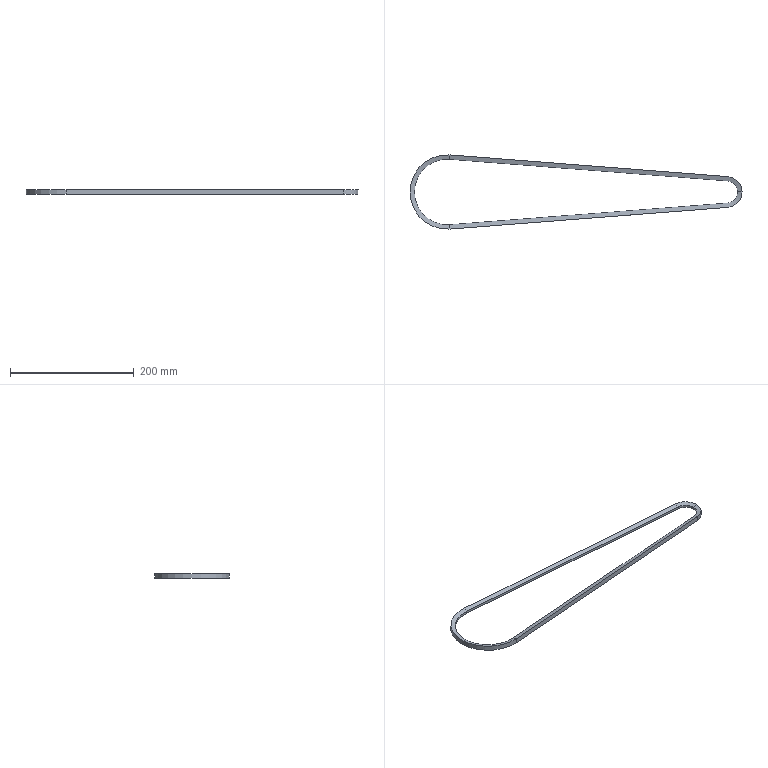Part | NX | features BREP 1 | 1 solid | 18 faces | box 535.87 x 119.96 x 8 mm | volume 48380 mm3 | plane 8 | cone 6 | cylinder 4 | commonest cylinder face diameters 35.96 x1 49.96 x1 105.96 x1 119.96 x1
STEP:
#1=CARTESIAN_POINT('',(4.112,52.82,-2.));
#2=VERTEX_POINT('',#1);
#3=CARTESIAN_POINT('',(-52.98,0.,-2.));
#4=VERTEX_POINT('',#3);
#5=CARTESIAN_POINT('',(0.,0.,-2.));
#6=DIRECTION('',(0.,0.,1.));
#7=DIRECTION('',(1.,0.,0.));
#8=AXIS2_PLACEMENT_3D('',#5,#6,#7);
#9=CIRCLE('',#8,52.98);
#10=EDGE_CURVE('',#2,#4,#9,.T.);
#11=ORIENTED_EDGE('',*,*,#10,.T.);
#12=CARTESIAN_POINT('',(-59.98,0.,-4.));
#13=VERTEX_POINT('',#12);
#14=CARTESIAN_POINT('',(-52.98,0.,-2.));
#15=DIRECTION('',(-0.9615,0.,-0.2747));
#16=VECTOR('',#15,1000.);
#17=LINE('',#14,#16);
#18=EDGE_CURVE('',#4,#13,#17,.T.);
#19=ORIENTED_EDGE('',*,*,#18,.T.);
#20=CARTESIAN_POINT('',(4.656,59.799,-4.));
#21=VERTEX_POINT('',#20);
#22=CARTESIAN_POINT('',(0.,0.,-4.));
#23=DIRECTION('',(0.,0.,1.));
#24=DIRECTION('',(1.,0.,0.));
#25=AXIS2_PLACEMENT_3D('',#22,#23,#24);
#26=CIRCLE('',#25,59.98);
#27=EDGE_CURVE('',#21,#13,#26,.T.);
#28=ORIENTED_EDGE('',*,*,#27,.F.);
#29=CARTESIAN_POINT('',(4.112,52.82,-2.));
#30=DIRECTION('',(0.07463,0.9586,-0.2747));
#31=VECTOR('',#30,1000.);
#32=LINE('',#29,#31);
#33=EDGE_CURVE('',#2,#21,#32,.T.);
#34=ORIENTED_EDGE('',*,*,#33,.F.);
#35=EDGE_LOOP('',(#11,#19,#28,#34));
#36=FACE_BOUND('',#35,.T.);
#37=CARTESIAN_POINT('',(0.,0.,-2.));
#38=DIRECTION('',(0.,0.,-1.));
#39=DIRECTION('',(1.,0.,0.));
#40=AXIS2_PLACEMENT_3D('',#37,#38,#39);
#41=CONICAL_SURFACE('',#40,52.98,1.292);
#42=ADVANCED_FACE('',(#36),#41,.F.);
#43=CARTESIAN_POINT('',(452.306,17.926,2.));
#44=VERTEX_POINT('',#43);
#45=CARTESIAN_POINT('',(468.89,0.,2.));
#46=VERTEX_POINT('',#45);
#47=CARTESIAN_POINT('',(450.91,0.,2.));
#48=DIRECTION('',(0.,0.,-1.));
#49=DIRECTION('',(-1.,0.,0.));
#50=AXIS2_PLACEMENT_3D('',#47,#48,#49);
#51=CIRCLE('',#50,17.98);
#52=EDGE_CURVE('',#44,#46,#51,.T.);
#53=ORIENTED_EDGE('',*,*,#52,.T.);
#54=CARTESIAN_POINT('',(475.89,0.,4.));
#55=VERTEX_POINT('',#54);
#56=CARTESIAN_POINT('',(475.89,0.,4.));
#57=DIRECTION('',(0.9615,0.,0.2747));
#58=VECTOR('',#57,1000.);
#59=LINE('',#56,#58);
#60=EDGE_CURVE('',#46,#55,#59,.T.);
#61=ORIENTED_EDGE('',*,*,#60,.T.);
#62=CARTESIAN_POINT('',(452.849,24.905,4.));
#63=VERTEX_POINT('',#62);
#64=CARTESIAN_POINT('',(450.91,0.,4.));
#65=DIRECTION('',(0.,0.,-1.));
#66=DIRECTION('',(-1.,0.,0.));
#67=AXIS2_PLACEMENT_3D('',#64,#65,#66);
#68=CIRCLE('',#67,24.98);
#69=EDGE_CURVE('',#63,#55,#68,.T.);
#70=ORIENTED_EDGE('',*,*,#69,.F.);
#71=CARTESIAN_POINT('',(452.306,17.926,2.));
#72=DIRECTION('',(-0.07463,-0.9586,-0.2747));
#73=VECTOR('',#72,1000.);
#74=LINE('',#71,#73);
#75=EDGE_CURVE('',#63,#44,#74,.T.);
#76=ORIENTED_EDGE('',*,*,#75,.T.);
#77=EDGE_LOOP('',(#53,#61,#70,#76));
#78=FACE_BOUND('',#77,.T.);
#79=CARTESIAN_POINT('',(450.91,0.,4.));
#80=DIRECTION('',(0.,0.,1.));
#81=DIRECTION('',(-1.,0.,0.));
#82=AXIS2_PLACEMENT_3D('',#79,#80,#81);
#83=CONICAL_SURFACE('',#82,24.98,1.292);
#84=ADVANCED_FACE('',(#78),#83,.F.);
#85=CARTESIAN_POINT('',(452.306,-17.926,2.));
#86=VERTEX_POINT('',#85);
#87=CARTESIAN_POINT('',(452.306,-17.926,-2.));
#88=VERTEX_POINT('',#87);
#89=CARTESIAN_POINT('',(452.306,-17.926,2.));
#90=DIRECTION('',(0.,0.,-1.));
#91=VECTOR('',#90,1000.);
#92=LINE('',#89,#91);
#93=EDGE_CURVE('',#86,#88,#92,.T.);
#94=ORIENTED_EDGE('',*,*,#93,.T.);
#95=CARTESIAN_POINT('',(4.112,-52.82,-2.));
#96=VERTEX_POINT('',#95);
#97=CARTESIAN_POINT('',(452.306,-17.926,-2.));
#98=DIRECTION('',(-0.997,-0.07762,0.));
#99=VECTOR('',#98,1000.);
#100=LINE('',#97,#99);
#101=EDGE_CURVE('',#88,#96,#100,.T.);
#102=ORIENTED_EDGE('',*,*,#101,.T.);
#103=CARTESIAN_POINT('',(4.112,-52.82,2.));
#104=VERTEX_POINT('',#103);
#105=CARTESIAN_POINT('',(4.112,-52.82,2.));
#106=DIRECTION('',(0.,0.,-1.));
#107=VECTOR('',#106,1000.);
#108=LINE('',#105,#107);
#109=EDGE_CURVE('',#104,#96,#108,.T.);
#110=ORIENTED_EDGE('',*,*,#109,.F.);
#111=CARTESIAN_POINT('',(452.306,-17.926,2.));
#112=DIRECTION('',(-0.997,-0.07762,0.));
#113=VECTOR('',#112,1000.);
#114=LINE('',#111,#113);
#115=EDGE_CURVE('',#86,#104,#114,.T.);
#116=ORIENTED_EDGE('',*,*,#115,.F.);
#117=EDGE_LOOP('',(#94,#102,#110,#116));
#118=FACE_BOUND('',#117,.T.);
#119=CARTESIAN_POINT('',(452.306,-17.926,2.));
#120=DIRECTION('',(-0.07762,0.997,0.));
#121=DIRECTION('',(0.,0.,-1.));
#122=AXIS2_PLACEMENT_3D('',#119,#120,#121);
#123=PLANE('',#122);
#124=ADVANCED_FACE('',(#118),#123,.T.);
#125=CARTESIAN_POINT('',(452.849,-24.905,-4.));
#126=VERTEX_POINT('',#125);
#127=CARTESIAN_POINT('',(452.306,-17.926,-2.));
#128=DIRECTION('',(0.07463,-0.9586,-0.2747));
#129=VECTOR('',#128,1000.);
#130=LINE('',#127,#129);
#131=EDGE_CURVE('',#88,#126,#130,.T.);
#132=ORIENTED_EDGE('',*,*,#131,.T.);
#133=CARTESIAN_POINT('',(4.656,-59.799,-4.));
#134=VERTEX_POINT('',#133);
#135=CARTESIAN_POINT('',(452.849,-24.905,-4.));
#136=DIRECTION('',(-0.997,-0.07762,0.));
#137=VECTOR('',#136,1000.);
#138=LINE('',#135,#137);
#139=EDGE_CURVE('',#126,#134,#138,.T.);
#140=ORIENTED_EDGE('',*,*,#139,.T.);
#141=CARTESIAN_POINT('',(4.112,-52.82,-2.));
#142=DIRECTION('',(0.07463,-0.9586,-0.2747));
#143=VECTOR('',#142,1000.);
#144=LINE('',#141,#143);
#145=EDGE_CURVE('',#96,#134,#144,.T.);
#146=ORIENTED_EDGE('',*,*,#145,.F.);
#147=ORIENTED_EDGE('',*,*,#101,.F.);
#148=EDGE_LOOP('',(#132,#140,#146,#147));
#149=FACE_BOUND('',#148,.T.);
#150=CARTESIAN_POINT('',(452.306,-17.926,-2.));
#151=DIRECTION('',(-0.02132,0.2739,-0.9615));
#152=DIRECTION('',(0.9998,0.,-0.02217));
#153=AXIS2_PLACEMENT_3D('',#150,#151,#152);
#154=PLANE('',#153);
#155=ADVANCED_FACE('',(#149),#154,.T.);
#156=CARTESIAN_POINT('',(452.849,-24.905,4.));
#157=VERTEX_POINT('',#156);
#158=CARTESIAN_POINT('',(452.849,-24.905,-4.));
#159=DIRECTION('',(0.,0.,1.));
#160=VECTOR('',#159,1000.);
#161=LINE('',#158,#160);
#162=EDGE_CURVE('',#126,#157,#161,.T.);
#163=ORIENTED_EDGE('',*,*,#162,.T.);
#164=CARTESIAN_POINT('',(4.656,-59.799,4.));
#165=VERTEX_POINT('',#164);
#166=CARTESIAN_POINT('',(452.849,-24.905,4.));
#167=DIRECTION('',(-0.997,-0.07762,0.));
#168=VECTOR('',#167,1000.);
#169=LINE('',#166,#168);
#170=EDGE_CURVE('',#157,#165,#169,.T.);
#171=ORIENTED_EDGE('',*,*,#170,.T.);
#172=CARTESIAN_POINT('',(4.656,-59.799,-4.));
#173=DIRECTION('',(0.,0.,1.));
#174=VECTOR('',#173,1000.);
#175=LINE('',#172,#174);
#176=EDGE_CURVE('',#134,#165,#175,.T.);
#177=ORIENTED_EDGE('',*,*,#176,.F.);
#178=ORIENTED_EDGE('',*,*,#139,.F.);
#179=EDGE_LOOP('',(#163,#171,#177,#178));
#180=FACE_BOUND('',#179,.T.);
#181=CARTESIAN_POINT('',(452.849,-24.905,-4.));
#182=DIRECTION('',(0.07762,-0.997,0.));
#183=DIRECTION('',(0.,0.,1.));
#184=AXIS2_PLACEMENT_3D('',#181,#182,#183);
#185=PLANE('',#184);
#186=ADVANCED_FACE('',(#180),#185,.T.);
#187=CARTESIAN_POINT('',(452.306,-17.926,2.));
#188=DIRECTION('',(-0.07463,0.9586,-0.2747));
#189=VECTOR('',#188,1000.);
#190=LINE('',#187,#189);
#191=EDGE_CURVE('',#157,#86,#190,.T.);
#192=ORIENTED_EDGE('',*,*,#191,.T.);
#193=ORIENTED_EDGE('',*,*,#115,.T.);
#194=CARTESIAN_POINT('',(4.112,-52.82,2.));
#195=DIRECTION('',(-0.07463,0.9586,-0.2747));
#196=VECTOR('',#195,1000.);
#197=LINE('',#194,#196);
#198=EDGE_CURVE('',#165,#104,#197,.T.);
#199=ORIENTED_EDGE('',*,*,#198,.F.);
#200=ORIENTED_EDGE('',*,*,#170,.F.);
#201=EDGE_LOOP('',(#192,#193,#199,#200));
#202=FACE_BOUND('',#201,.T.);
#203=CARTESIAN_POINT('',(452.306,-17.926,2.));
#204=DIRECTION('',(-0.02132,0.2739,0.9615));
#205=DIRECTION('',(-0.997,-0.07762,0.));
#206=AXIS2_PLACEMENT_3D('',#203,#204,#205);
#207=PLANE('',#206);
#208=ADVANCED_FACE('',(#202),#207,.T.);
#209=CARTESIAN_POINT('',(452.306,17.926,-2.));
#210=VERTEX_POINT('',#209);
#211=CARTESIAN_POINT('',(452.306,17.926,2.));
#212=DIRECTION('',(0.,0.,-1.));
#213=VECTOR('',#212,1000.);
#214=LINE('',#211,#213);
#215=EDGE_CURVE('',#44,#210,#214,.T.);
#216=ORIENTED_EDGE('',*,*,#215,.T.);
#217=CARTESIAN_POINT('',(450.91,0.,-2.));
#218=DIRECTION('',(0.,0.,-1.));
#219=DIRECTION('',(-1.,0.,0.));
#220=AXIS2_PLACEMENT_3D('',#217,#218,#219);
#221=CIRCLE('',#220,17.98);
#222=EDGE_CURVE('',#210,#88,#221,.T.);
#223=ORIENTED_EDGE('',*,*,#222,.T.);
#224=ORIENTED_EDGE('',*,*,#93,.F.);
#225=CARTESIAN_POINT('',(450.91,0.,2.));
#226=DIRECTION('',(0.,0.,-1.));
#227=DIRECTION('',(-1.,0.,0.));
#228=AXIS2_PLACEMENT_3D('',#225,#226,#227);
#229=CIRCLE('',#228,17.98);
#230=EDGE_CURVE('',#46,#86,#229,.T.);
#231=ORIENTED_EDGE('',*,*,#230,.F.);
#232=ORIENTED_EDGE('',*,*,#52,.F.);
#233=EDGE_LOOP('',(#216,#223,#224,#231,#232));
#234=FACE_BOUND('',#233,.T.);
#235=CARTESIAN_POINT('',(450.91,0.,0.));
#236=DIRECTION('',(0.,0.,-1.));
#237=DIRECTION('',(1.,0.,0.));
#238=AXIS2_PLACEMENT_3D('',#235,#236,#237);
#239=CYLINDRICAL_SURFACE('',#238,17.98);
#240=ADVANCED_FACE('',(#234),#239,.F.);
#241=CARTESIAN_POINT('',(452.849,24.905,-4.));
#242=VERTEX_POINT('',#241);
#243=CARTESIAN_POINT('',(452.306,17.926,-2.));
#244=DIRECTION('',(0.07463,0.9586,-0.2747));
#245=VECTOR('',#244,1000.);
#246=LINE('',#243,#245);
#247=EDGE_CURVE('',#210,#242,#246,.T.);
#248=ORIENTED_EDGE('',*,*,#247,.T.);
#249=CARTESIAN_POINT('',(450.91,0.,-4.));
#250=DIRECTION('',(0.,0.,-1.));
#251=DIRECTION('',(-1.,0.,0.));
#252=AXIS2_PLACEMENT_3D('',#249,#250,#251);
#253=CIRCLE('',#252,24.98);
#254=EDGE_CURVE('',#242,#126,#253,.T.);
#255=ORIENTED_EDGE('',*,*,#254,.T.);
#256=ORIENTED_EDGE('',*,*,#131,.F.);
#257=ORIENTED_EDGE('',*,*,#222,.F.);
#258=EDGE_LOOP('',(#248,#255,#256,#257));
#259=FACE_BOUND('',#258,.T.);
#260=CARTESIAN_POINT('',(450.91,0.,-2.));
#261=DIRECTION('',(0.,0.,-1.));
#262=DIRECTION('',(1.,0.,0.));
#263=AXIS2_PLACEMENT_3D('',#260,#261,#262);
#264=CONICAL_SURFACE('',#263,17.98,1.292);
#265=ADVANCED_FACE('',(#259),#264,.F.);
#266=CARTESIAN_POINT('',(452.849,24.905,-4.));
#267=DIRECTION('',(0.,0.,1.));
#268=VECTOR('',#267,1000.);
#269=LINE('',#266,#268);
#270=EDGE_CURVE('',#242,#63,#269,.T.);
#271=ORIENTED_EDGE('',*,*,#270,.T.);
#272=ORIENTED_EDGE('',*,*,#69,.T.);
#273=CARTESIAN_POINT('',(450.91,0.,4.));
#274=DIRECTION('',(0.,0.,-1.));
#275=DIRECTION('',(-1.,0.,0.));
#276=AXIS2_PLACEMENT_3D('',#273,#274,#275);
#277=CIRCLE('',#276,24.98);
#278=EDGE_CURVE('',#55,#157,#277,.T.);
#279=ORIENTED_EDGE('',*,*,#278,.T.);
#280=ORIENTED_EDGE('',*,*,#162,.F.);
#281=ORIENTED_EDGE('',*,*,#254,.F.);
#282=EDGE_LOOP('',(#271,#272,#279,#280,#281));
#283=FACE_BOUND('',#282,.T.);
#284=CARTESIAN_POINT('',(450.91,0.,0.));
#285=DIRECTION('',(0.,0.,-1.));
#286=DIRECTION('',(1.,0.,0.));
#287=AXIS2_PLACEMENT_3D('',#284,#285,#286);
#288=CYLINDRICAL_SURFACE('',#287,24.98);
#289=ADVANCED_FACE('',(#283),#288,.T.);
#290=ORIENTED_EDGE('',*,*,#60,.F.);
#291=ORIENTED_EDGE('',*,*,#230,.T.);
#292=ORIENTED_EDGE('',*,*,#191,.F.);
#293=ORIENTED_EDGE('',*,*,#278,.F.);
#294=EDGE_LOOP('',(#290,#291,#292,#293));
#295=FACE_BOUND('',#294,.T.);
#296=CARTESIAN_POINT('',(450.91,0.,4.));
#297=DIRECTION('',(0.,0.,1.));
#298=DIRECTION('',(-1.,0.,0.));
#299=AXIS2_PLACEMENT_3D('',#296,#297,#298);
#300=CONICAL_SURFACE('',#299,24.98,1.292);
#301=ADVANCED_FACE('',(#295),#300,.F.);
#302=CARTESIAN_POINT('',(4.112,52.82,2.));
#303=VERTEX_POINT('',#302);
#304=CARTESIAN_POINT('',(4.112,52.82,2.));
#305=DIRECTION('',(0.,0.,-1.));
#306=VECTOR('',#305,1000.);
#307=LINE('',#304,#306);
#308=EDGE_CURVE('',#303,#2,#307,.T.);
#309=ORIENTED_EDGE('',*,*,#308,.T.);
#310=CARTESIAN_POINT('',(4.112,52.82,-2.));
#311=DIRECTION('',(0.997,-0.07762,0.));
#312=VECTOR('',#311,1000.);
#313=LINE('',#310,#312);
#314=EDGE_CURVE('',#2,#210,#313,.T.);
#315=ORIENTED_EDGE('',*,*,#314,.T.);
#316=ORIENTED_EDGE('',*,*,#215,.F.);
#317=CARTESIAN_POINT('',(4.112,52.82,2.));
#318=DIRECTION('',(0.997,-0.07762,0.));
#319=VECTOR('',#318,1000.);
#320=LINE('',#317,#319);
#321=EDGE_CURVE('',#303,#44,#320,.T.);
#322=ORIENTED_EDGE('',*,*,#321,.F.);
#323=EDGE_LOOP('',(#309,#315,#316,#322));
#324=FACE_BOUND('',#323,.T.);
#325=CARTESIAN_POINT('',(4.112,52.82,2.));
#326=DIRECTION('',(-0.07762,-0.997,0.));
#327=DIRECTION('',(0.997,-0.07762,0.));
#328=AXIS2_PLACEMENT_3D('',#325,#326,#327);
#329=PLANE('',#328);
#330=ADVANCED_FACE('',(#324),#329,.T.);
#331=ORIENTED_EDGE('',*,*,#33,.T.);
#332=CARTESIAN_POINT('',(4.656,59.799,-4.));
#333=DIRECTION('',(0.997,-0.07762,0.));
#334=VECTOR('',#333,1000.);
#335=LINE('',#332,#334);
#336=EDGE_CURVE('',#21,#242,#335,.T.);
#337=ORIENTED_EDGE('',*,*,#336,.T.);
#338=ORIENTED_EDGE('',*,*,#247,.F.);
#339=ORIENTED_EDGE('',*,*,#314,.F.);
#340=EDGE_LOOP('',(#331,#337,#338,#339));
#341=FACE_BOUND('',#340,.T.);
#342=CARTESIAN_POINT('',(4.112,52.82,-2.));
#343=DIRECTION('',(-0.02132,-0.2739,-0.9615));
#344=DIRECTION('',(0.,0.9617,-0.274));
#345=AXIS2_PLACEMENT_3D('',#342,#343,#344);
#346=PLANE('',#345);
#347=ADVANCED_FACE('',(#341),#346,.T.);
#348=CARTESIAN_POINT('',(4.656,59.799,4.));
#349=VERTEX_POINT('',#348);
#350=CARTESIAN_POINT('',(4.656,59.799,-4.));
#351=DIRECTION('',(0.,0.,1.));
#352=VECTOR('',#351,1000.);
#353=LINE('',#350,#352);
#354=EDGE_CURVE('',#21,#349,#353,.T.);
#355=ORIENTED_EDGE('',*,*,#354,.T.);
#356=CARTESIAN_POINT('',(4.656,59.799,4.));
#357=DIRECTION('',(0.997,-0.07762,0.));
#358=VECTOR('',#357,1000.);
#359=LINE('',#356,#358);
#360=EDGE_CURVE('',#349,#63,#359,.T.);
#361=ORIENTED_EDGE('',*,*,#360,.T.);
#362=ORIENTED_EDGE('',*,*,#270,.F.);
#363=ORIENTED_EDGE('',*,*,#336,.F.);
#364=EDGE_LOOP('',(#355,#361,#362,#363));
#365=FACE_BOUND('',#364,.T.);
#366=CARTESIAN_POINT('',(4.656,59.799,-4.));
#367=DIRECTION('',(0.07762,0.997,0.));
#368=DIRECTION('',(0.,0.,1.));
#369=AXIS2_PLACEMENT_3D('',#366,#367,#368);
#370=PLANE('',#369);
#371=ADVANCED_FACE('',(#365),#370,.T.);
#372=CARTESIAN_POINT('',(4.112,52.82,2.));
#373=DIRECTION('',(-0.07463,-0.9586,-0.2747));
#374=VECTOR('',#373,1000.);
#375=LINE('',#372,#374);
#376=EDGE_CURVE('',#349,#303,#375,.T.);
#377=ORIENTED_EDGE('',*,*,#376,.T.);
#378=ORIENTED_EDGE('',*,*,#321,.T.);
#379=ORIENTED_EDGE('',*,*,#75,.F.);
#380=ORIENTED_EDGE('',*,*,#360,.F.);
#381=EDGE_LOOP('',(#377,#378,#379,#380));
#382=FACE_BOUND('',#381,.T.);
#383=CARTESIAN_POINT('',(4.112,52.82,2.));
#384=DIRECTION('',(-0.02132,-0.2739,0.9615));
#385=DIRECTION('',(0.997,-0.07762,0.));
#386=AXIS2_PLACEMENT_3D('',#383,#384,#385);
#387=PLANE('',#386);
#388=ADVANCED_FACE('',(#382),#387,.T.);
#389=CARTESIAN_POINT('',(0.,0.,2.));
#390=DIRECTION('',(0.,0.,1.));
#391=DIRECTION('',(1.,0.,0.));
#392=AXIS2_PLACEMENT_3D('',#389,#390,#391);
#393=CIRCLE('',#392,52.98);
#394=EDGE_CURVE('',#303,#104,#393,.T.);
#395=ORIENTED_EDGE('',*,*,#394,.F.);
#396=ORIENTED_EDGE('',*,*,#376,.F.);
#397=CARTESIAN_POINT('',(0.,0.,4.));
#398=DIRECTION('',(0.,0.,1.));
#399=DIRECTION('',(1.,0.,0.));
#400=AXIS2_PLACEMENT_3D('',#397,#398,#399);
#401=CIRCLE('',#400,59.98);
#402=EDGE_CURVE('',#349,#165,#401,.T.);
#403=ORIENTED_EDGE('',*,*,#402,.T.);
#404=ORIENTED_EDGE('',*,*,#198,.T.);
#405=EDGE_LOOP('',(#395,#396,#403,#404));
#406=FACE_BOUND('',#405,.T.);
#407=CARTESIAN_POINT('',(0.,0.,4.));
#408=DIRECTION('',(0.,0.,1.));
#409=DIRECTION('',(-1.,0.,0.));
#410=AXIS2_PLACEMENT_3D('',#407,#408,#409);
#411=CONICAL_SURFACE('',#410,59.98,1.292);
#412=ADVANCED_FACE('',(#406),#411,.F.);
#413=ORIENTED_EDGE('',*,*,#10,.F.);
#414=ORIENTED_EDGE('',*,*,#308,.F.);
#415=ORIENTED_EDGE('',*,*,#394,.T.);
#416=ORIENTED_EDGE('',*,*,#109,.T.);
#417=CARTESIAN_POINT('',(0.,0.,-2.));
#418=DIRECTION('',(0.,0.,1.));
#419=DIRECTION('',(1.,0.,0.));
#420=AXIS2_PLACEMENT_3D('',#417,#418,#419);
#421=CIRCLE('',#420,52.98);
#422=EDGE_CURVE('',#4,#96,#421,.T.);
#423=ORIENTED_EDGE('',*,*,#422,.F.);
#424=EDGE_LOOP('',(#413,#414,#415,#416,#423));
#425=FACE_BOUND('',#424,.T.);
#426=CARTESIAN_POINT('',(0.,0.,0.));
#427=DIRECTION('',(0.,0.,1.));
#428=DIRECTION('',(-1.,0.,0.));
#429=AXIS2_PLACEMENT_3D('',#426,#427,#428);
#430=CYLINDRICAL_SURFACE('',#429,52.98);
#431=ADVANCED_FACE('',(#425),#430,.F.);
#432=ORIENTED_EDGE('',*,*,#18,.F.);
#433=ORIENTED_EDGE('',*,*,#422,.T.);
#434=ORIENTED_EDGE('',*,*,#145,.T.);
#435=CARTESIAN_POINT('',(0.,0.,-4.));
#436=DIRECTION('',(0.,0.,1.));
#437=DIRECTION('',(1.,0.,0.));
#438=AXIS2_PLACEMENT_3D('',#435,#436,#437);
#439=CIRCLE('',#438,59.98);
#440=EDGE_CURVE('',#13,#134,#439,.T.);
#441=ORIENTED_EDGE('',*,*,#440,.F.);
#442=EDGE_LOOP('',(#432,#433,#434,#441));
#443=FACE_BOUND('',#442,.T.);
#444=CARTESIAN_POINT('',(0.,0.,-2.));
#445=DIRECTION('',(0.,0.,-1.));
#446=DIRECTION('',(1.,0.,0.));
#447=AXIS2_PLACEMENT_3D('',#444,#445,#446);
#448=CONICAL_SURFACE('',#447,52.98,1.292);
#449=ADVANCED_FACE('',(#443),#448,.F.);
#450=ORIENTED_EDGE('',*,*,#354,.F.);
#451=ORIENTED_EDGE('',*,*,#27,.T.);
#452=ORIENTED_EDGE('',*,*,#440,.T.);
#453=ORIENTED_EDGE('',*,*,#176,.T.);
#454=ORIENTED_EDGE('',*,*,#402,.F.);
#455=EDGE_LOOP('',(#450,#451,#452,#453,#454));
#456=FACE_BOUND('',#455,.T.);
#457=CARTESIAN_POINT('',(0.,0.,0.));
#458=DIRECTION('',(0.,0.,1.));
#459=DIRECTION('',(-1.,0.,0.));
#460=AXIS2_PLACEMENT_3D('',#457,#458,#459);
#461=CYLINDRICAL_SURFACE('',#460,59.98);
#462=ADVANCED_FACE('',(#456),#461,.T.);
#463=CLOSED_SHELL('',(#42,#84,#124,#155,#186,#208,#240,#265,#289,#301,#330,#347,#371,#388,#412,#431,#449,#462));
#464=MANIFOLD_SOLID_BREP('',#463);
#465=(LENGTH_UNIT()NAMED_UNIT(*)SI_UNIT(.MILLI.,.METRE.));
#466=UNCERTAINTY_MEASURE_WITH_UNIT(LENGTH_MEASURE(0.00001),#465,'','');
#467=(NAMED_UNIT(*)PLANE_ANGLE_UNIT()SI_UNIT($,.RADIAN.));
#468=(NAMED_UNIT(*)SI_UNIT($,.STERADIAN.)SOLID_ANGLE_UNIT());
#469=(GEOMETRIC_REPRESENTATION_CONTEXT(3)GLOBAL_UNCERTAINTY_ASSIGNED_CONTEXT((#466))GLOBAL_UNIT_ASSIGNED_CONTEXT((#465,#467,#468))REPRESENTATION_CONTEXT('',''));
#470=ADVANCED_BREP_SHAPE_REPRESENTATION('',(#464),#469);